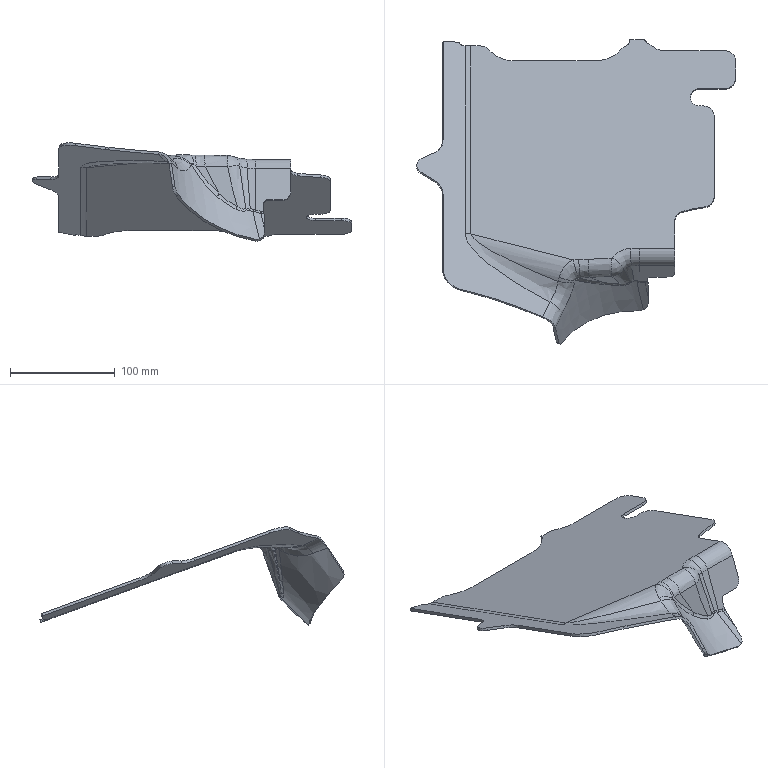Part | STEP file | lll_id30_x_t | 1 solid | 129 faces | box 304.48 x 290.044 x 93.8 mm | volume 170450 mm3 | spline 81 | plane 32 | cylinder 14 | torus 2 | commonest cylinder face diameters 1 x4 55 x2 21 x1 26 x1 50 x1 60 x1